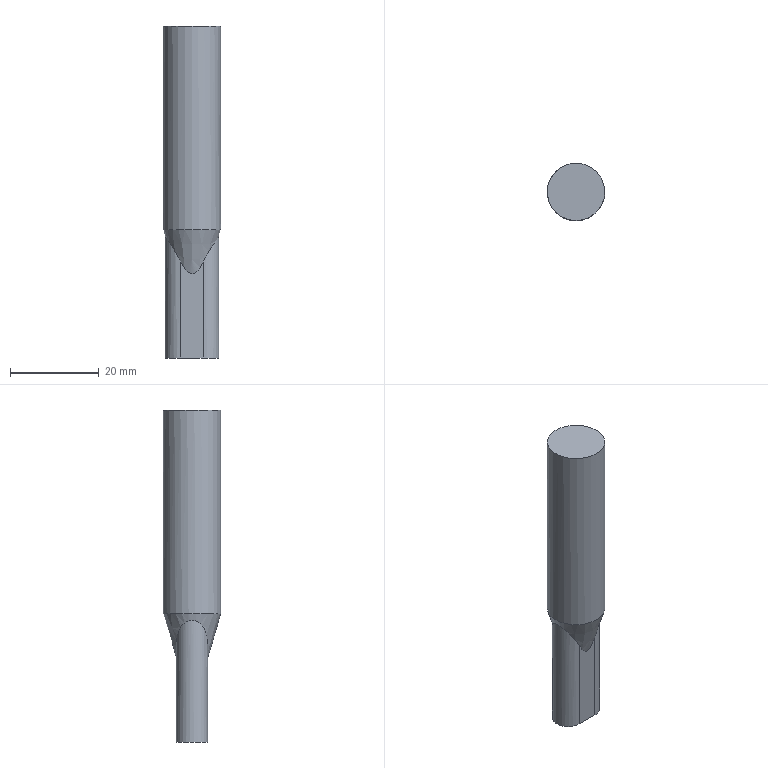Part | NX | features solid 2 | 1 solid | 8 faces | box 13 x 13 x 75 mm | volume 8475 mm3 | plane 4 | cylinder 3 | cone 1 | commonest cylinder face diameters 7.1 x2 13 x1
STEP:
#1=CARTESIAN_POINT('',(-220.46,-80.652,68.685));
#2=VERTEX_POINT('',#1);
#3=CARTESIAN_POINT('',(-225.46,-80.652,68.685));
#4=VERTEX_POINT('',#3);
#5=CARTESIAN_POINT('',(-225.46,-80.652,68.685));
#6=CARTESIAN_POINT('',(-225.174,-80.652,68.125));
#7=CARTESIAN_POINT('',(-224.706,-80.652,67.297));
#8=CARTESIAN_POINT('',(-223.883,-80.652,66.312));
#9=CARTESIAN_POINT('',(-222.957,-80.652,65.843));
#10=CARTESIAN_POINT('',(-222.035,-80.652,66.316));
#11=CARTESIAN_POINT('',(-221.218,-80.652,67.294));
#12=CARTESIAN_POINT('',(-220.749,-80.652,68.121));
#13=CARTESIAN_POINT('',(-220.46,-80.652,68.685));
#14=B_SPLINE_CURVE_WITH_KNOTS('',3,(#5,#6,#7,#8,#9,#10,#11,#12,#13),.UNSPECIFIED.,.F.,.F.,(4,1,1,1,1,1,4),(0.02112,0.02301,0.02395,0.0249,0.02584,0.02679,0.02868),.UNSPECIFIED.);
#15=EDGE_CURVE('',#2,#4,#14,.F.);
#16=ORIENTED_EDGE('',*,*,#15,.F.);
#17=CARTESIAN_POINT('',(-220.46,-80.652,47.));
#18=VERTEX_POINT('',#17);
#19=CARTESIAN_POINT('',(-220.46,-80.652,47.));
#20=DIRECTION('',(0.,0.,1.));
#21=VECTOR('',#20,1000.);
#22=LINE('',#19,#21);
#23=EDGE_CURVE('',#18,#2,#22,.T.);
#24=ORIENTED_EDGE('',*,*,#23,.F.);
#25=CARTESIAN_POINT('',(-225.46,-80.652,47.));
#26=VERTEX_POINT('',#25);
#27=CARTESIAN_POINT('',(-222.96,-80.652,47.));
#28=DIRECTION('',(-1.,0.,0.));
#29=VECTOR('',#28,1000.);
#30=LINE('',#27,#29);
#31=EDGE_CURVE('',#18,#26,#30,.T.);
#32=ORIENTED_EDGE('',*,*,#31,.T.);
#33=CARTESIAN_POINT('',(-225.46,-80.652,47.));
#34=DIRECTION('',(0.,0.,1.));
#35=VECTOR('',#34,1000.);
#36=LINE('',#33,#35);
#37=EDGE_CURVE('',#26,#4,#36,.T.);
#38=ORIENTED_EDGE('',*,*,#37,.T.);
#39=EDGE_LOOP('',(#16,#24,#32,#38));
#40=FACE_BOUND('',#39,.T.);
#41=CARTESIAN_POINT('',(-222.96,-80.652,47.));
#42=DIRECTION('',(0.,1.,0.));
#43=DIRECTION('',(0.,0.,1.));
#44=AXIS2_PLACEMENT_3D('',#41,#42,#43);
#45=PLANE('',#44);
#46=ADVANCED_FACE('',(#40),#45,.T.);
#47=ORIENTED_EDGE('',*,*,#31,.F.);
#48=CARTESIAN_POINT('',(-220.46,-87.752,47.));
#49=VERTEX_POINT('',#48);
#50=CARTESIAN_POINT('',(-220.46,-84.202,47.));
#51=DIRECTION('',(0.,0.,1.));
#52=DIRECTION('',(0.,-1.,0.));
#53=AXIS2_PLACEMENT_3D('',#50,#51,#52);
#54=CIRCLE('',#53,3.55);
#55=EDGE_CURVE('',#49,#18,#54,.T.);
#56=ORIENTED_EDGE('',*,*,#55,.F.);
#57=CARTESIAN_POINT('',(-225.46,-87.752,47.));
#58=VERTEX_POINT('',#57);
#59=CARTESIAN_POINT('',(-222.96,-87.752,47.));
#60=DIRECTION('',(1.,0.,0.));
#61=VECTOR('',#60,1000.);
#62=LINE('',#59,#61);
#63=EDGE_CURVE('',#58,#49,#62,.T.);
#64=ORIENTED_EDGE('',*,*,#63,.F.);
#65=CARTESIAN_POINT('',(-225.46,-84.202,47.));
#66=DIRECTION('',(0.,0.,1.));
#67=DIRECTION('',(0.,-1.,0.));
#68=AXIS2_PLACEMENT_3D('',#65,#66,#67);
#69=CIRCLE('',#68,3.55);
#70=EDGE_CURVE('',#26,#58,#69,.T.);
#71=ORIENTED_EDGE('',*,*,#70,.F.);
#72=EDGE_LOOP('',(#47,#56,#64,#71));
#73=FACE_BOUND('',#72,.T.);
#74=CARTESIAN_POINT('',(-222.96,-84.202,47.));
#75=DIRECTION('',(0.,0.,-1.));
#76=DIRECTION('',(0.,1.,0.));
#77=AXIS2_PLACEMENT_3D('',#74,#75,#76);
#78=PLANE('',#77);
#79=ADVANCED_FACE('',(#73),#78,.T.);
#80=CARTESIAN_POINT('',(-225.46,-87.752,68.685));
#81=VERTEX_POINT('',#80);
#82=CARTESIAN_POINT('',(-220.46,-87.752,68.685));
#83=VERTEX_POINT('',#82);
#84=CARTESIAN_POINT('',(-225.46,-87.752,68.685));
#85=CARTESIAN_POINT('',(-225.174,-87.752,68.125));
#86=CARTESIAN_POINT('',(-224.706,-87.752,67.297));
#87=CARTESIAN_POINT('',(-223.883,-87.752,66.312));
#88=CARTESIAN_POINT('',(-222.957,-87.752,65.843));
#89=CARTESIAN_POINT('',(-222.035,-87.752,66.316));
#90=CARTESIAN_POINT('',(-221.218,-87.752,67.294));
#91=CARTESIAN_POINT('',(-220.749,-87.752,68.121));
#92=CARTESIAN_POINT('',(-220.46,-87.752,68.685));
#93=B_SPLINE_CURVE_WITH_KNOTS('',3,(#84,#85,#86,#87,#88,#89,#90,#91,#92),.UNSPECIFIED.,.F.,.F.,(4,1,1,1,1,1,4),(0.02112,0.02301,0.02395,0.0249,0.02584,0.02679,0.02868),.UNSPECIFIED.);
#94=EDGE_CURVE('',#81,#83,#93,.T.);
#95=ORIENTED_EDGE('',*,*,#94,.F.);
#96=CARTESIAN_POINT('',(-225.46,-87.752,47.));
#97=DIRECTION('',(0.,0.,1.));
#98=VECTOR('',#97,1000.);
#99=LINE('',#96,#98);
#100=EDGE_CURVE('',#58,#81,#99,.T.);
#101=ORIENTED_EDGE('',*,*,#100,.F.);
#102=ORIENTED_EDGE('',*,*,#63,.T.);
#103=CARTESIAN_POINT('',(-220.46,-87.752,47.));
#104=DIRECTION('',(0.,0.,1.));
#105=VECTOR('',#104,1000.);
#106=LINE('',#103,#105);
#107=EDGE_CURVE('',#49,#83,#106,.T.);
#108=ORIENTED_EDGE('',*,*,#107,.T.);
#109=EDGE_LOOP('',(#95,#101,#102,#108));
#110=FACE_BOUND('',#109,.T.);
#111=CARTESIAN_POINT('',(-222.96,-87.752,47.));
#112=DIRECTION('',(0.,-1.,0.));
#113=DIRECTION('',(0.,0.,-1.));
#114=AXIS2_PLACEMENT_3D('',#111,#112,#113);
#115=PLANE('',#114);
#116=ADVANCED_FACE('',(#110),#115,.T.);
#117=CARTESIAN_POINT('',(-220.46,-80.652,68.685));
#118=CARTESIAN_POINT('',(-220.147,-80.652,69.296));
#119=CARTESIAN_POINT('',(-219.488,-80.734,70.506));
#120=CARTESIAN_POINT('',(-218.426,-81.204,72.254));
#121=CARTESIAN_POINT('',(-217.552,-82.034,73.563));
#122=CARTESIAN_POINT('',(-217.027,-83.131,74.312));
#123=CARTESIAN_POINT('',(-216.855,-84.184,74.552));
#124=CARTESIAN_POINT('',(-217.016,-85.238,74.327));
#125=CARTESIAN_POINT('',(-217.534,-86.348,73.59));
#126=CARTESIAN_POINT('',(-218.413,-87.192,72.276));
#127=CARTESIAN_POINT('',(-219.47,-87.667,70.537));
#128=CARTESIAN_POINT('',(-220.144,-87.752,69.303));
#129=CARTESIAN_POINT('',(-220.46,-87.752,68.685));
#130=B_SPLINE_CURVE_WITH_KNOTS('',3,(#117,#118,#119,#120,#121,#122,#123,#124,#125,#126,#127,#128,#129),.UNSPECIFIED.,.F.,.F.,(4,1,1,1,1,1,1,1,1,1,4),(0.002959,0.00502,0.00708,0.00914,0.01017,0.0112,0.01223,0.01326,0.01532,0.01738,0.01944),.UNSPECIFIED.);
#131=EDGE_CURVE('',#2,#83,#130,.T.);
#132=ORIENTED_EDGE('',*,*,#131,.F.);
#133=ORIENTED_EDGE('',*,*,#15,.T.);
#134=CARTESIAN_POINT('',(-225.46,-87.752,68.685));
#135=CARTESIAN_POINT('',(-225.774,-87.752,69.296));
#136=CARTESIAN_POINT('',(-226.433,-87.671,70.506));
#137=CARTESIAN_POINT('',(-227.495,-87.201,72.254));
#138=CARTESIAN_POINT('',(-228.369,-86.371,73.563));
#139=CARTESIAN_POINT('',(-228.894,-85.274,74.312));
#140=CARTESIAN_POINT('',(-229.066,-84.221,74.552));
#141=CARTESIAN_POINT('',(-228.905,-83.167,74.327));
#142=CARTESIAN_POINT('',(-228.387,-82.057,73.59));
#143=CARTESIAN_POINT('',(-227.508,-81.213,72.276));
#144=CARTESIAN_POINT('',(-226.451,-80.738,70.537));
#145=CARTESIAN_POINT('',(-225.777,-80.652,69.303));
#146=CARTESIAN_POINT('',(-225.46,-80.652,68.685));
#147=B_SPLINE_CURVE_WITH_KNOTS('',3,(#134,#135,#136,#137,#138,#139,#140,#141,#142,#143,#144,#145,#146),.UNSPECIFIED.,.F.,.F.,(4,1,1,1,1,1,1,1,1,1,4),(0.002959,0.00502,0.00708,0.00914,0.01017,0.0112,0.01223,0.01326,0.01532,0.01738,0.01944),.UNSPECIFIED.);
#148=EDGE_CURVE('',#81,#4,#147,.T.);
#149=ORIENTED_EDGE('',*,*,#148,.F.);
#150=ORIENTED_EDGE('',*,*,#94,.T.);
#151=EDGE_LOOP('',(#132,#133,#149,#150));
#152=FACE_BOUND('',#151,.T.);
#153=CARTESIAN_POINT('',(-222.96,-90.702,76.));
#154=VERTEX_POINT('',#153);
#155=CARTESIAN_POINT('',(-222.96,-84.202,76.));
#156=DIRECTION('',(0.,0.,1.));
#157=DIRECTION('',(0.,-1.,0.));
#158=AXIS2_PLACEMENT_3D('',#155,#156,#157);
#159=CIRCLE('',#158,6.5);
#160=EDGE_CURVE('',#154,#154,#159,.T.);
#161=ORIENTED_EDGE('',*,*,#160,.F.);
#162=EDGE_LOOP('',(#161));
#163=FACE_BOUND('',#162,.T.);
#164=CARTESIAN_POINT('',(-222.96,-84.202,66.));
#165=DIRECTION('',(0.,0.,1.));
#166=DIRECTION('',(0.,-1.,0.));
#167=AXIS2_PLACEMENT_3D('',#164,#165,#166);
#168=CONICAL_SURFACE('',#167,3.55,0.2869);
#169=ADVANCED_FACE('',(#152,#163),#168,.T.);
#170=CARTESIAN_POINT('',(-216.46,-84.202,122.));
#171=VERTEX_POINT('',#170);
#172=CARTESIAN_POINT('',(-222.96,-84.202,122.));
#173=DIRECTION('',(0.,0.,1.));
#174=DIRECTION('',(1.,0.,0.));
#175=AXIS2_PLACEMENT_3D('',#172,#173,#174);
#176=CIRCLE('',#175,6.5);
#177=EDGE_CURVE('',#171,#171,#176,.F.);
#178=ORIENTED_EDGE('',*,*,#177,.F.);
#179=EDGE_LOOP('',(#178));
#180=FACE_BOUND('',#179,.T.);
#181=CARTESIAN_POINT('',(-222.96,-84.202,122.));
#182=DIRECTION('',(0.,0.,1.));
#183=DIRECTION('',(0.,-1.,0.));
#184=AXIS2_PLACEMENT_3D('',#181,#182,#183);
#185=PLANE('',#184);
#186=ADVANCED_FACE('',(#180),#185,.T.);
#187=ORIENTED_EDGE('',*,*,#177,.T.);
#188=EDGE_LOOP('',(#187));
#189=FACE_BOUND('',#188,.T.);
#190=ORIENTED_EDGE('',*,*,#160,.T.);
#191=EDGE_LOOP('',(#190));
#192=FACE_BOUND('',#191,.T.);
#193=CARTESIAN_POINT('',(-222.96,-84.202,76.));
#194=DIRECTION('',(0.,0.,1.));
#195=DIRECTION('',(0.,-1.,0.));
#196=AXIS2_PLACEMENT_3D('',#193,#194,#195);
#197=CYLINDRICAL_SURFACE('',#196,6.5);
#198=ADVANCED_FACE('',(#189,#192),#197,.T.);
#199=ORIENTED_EDGE('',*,*,#37,.F.);
#200=ORIENTED_EDGE('',*,*,#70,.T.);
#201=ORIENTED_EDGE('',*,*,#100,.T.);
#202=ORIENTED_EDGE('',*,*,#148,.T.);
#203=EDGE_LOOP('',(#199,#200,#201,#202));
#204=FACE_BOUND('',#203,.T.);
#205=CARTESIAN_POINT('',(-225.46,-84.202,47.));
#206=DIRECTION('',(0.,0.,1.));
#207=DIRECTION('',(0.,-1.,0.));
#208=AXIS2_PLACEMENT_3D('',#205,#206,#207);
#209=CYLINDRICAL_SURFACE('',#208,3.55);
#210=ADVANCED_FACE('',(#204),#209,.T.);
#211=ORIENTED_EDGE('',*,*,#55,.T.);
#212=ORIENTED_EDGE('',*,*,#23,.T.);
#213=ORIENTED_EDGE('',*,*,#131,.T.);
#214=ORIENTED_EDGE('',*,*,#107,.F.);
#215=EDGE_LOOP('',(#211,#212,#213,#214));
#216=FACE_BOUND('',#215,.T.);
#217=CARTESIAN_POINT('',(-220.46,-84.202,47.));
#218=DIRECTION('',(0.,0.,1.));
#219=DIRECTION('',(0.,-1.,0.));
#220=AXIS2_PLACEMENT_3D('',#217,#218,#219);
#221=CYLINDRICAL_SURFACE('',#220,3.55);
#222=ADVANCED_FACE('',(#216),#221,.T.);
#223=CLOSED_SHELL('',(#46,#79,#116,#169,#186,#198,#210,#222));
#224=MANIFOLD_SOLID_BREP('',#223);
#225=(LENGTH_UNIT()NAMED_UNIT(*)SI_UNIT(.MILLI.,.METRE.));
#226=UNCERTAINTY_MEASURE_WITH_UNIT(LENGTH_MEASURE(0.0508),#225,'','');
#227=(NAMED_UNIT(*)PLANE_ANGLE_UNIT()SI_UNIT($,.RADIAN.));
#228=(NAMED_UNIT(*)SI_UNIT($,.STERADIAN.)SOLID_ANGLE_UNIT());
#229=(GEOMETRIC_REPRESENTATION_CONTEXT(3)GLOBAL_UNCERTAINTY_ASSIGNED_CONTEXT((#226))GLOBAL_UNIT_ASSIGNED_CONTEXT((#225,#227,#228))REPRESENTATION_CONTEXT('',''));
#230=ADVANCED_BREP_SHAPE_REPRESENTATION('',(#224),#229);